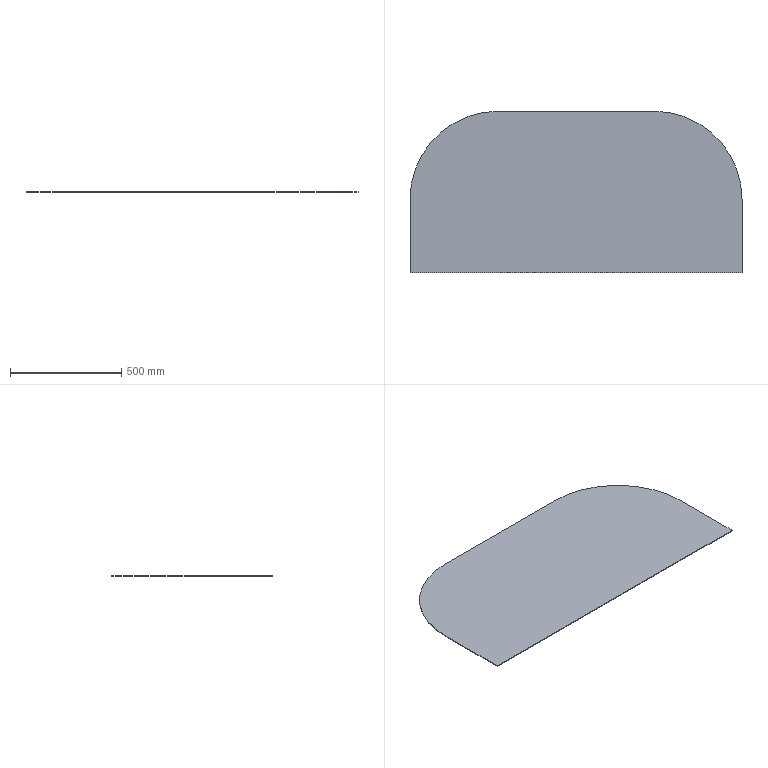Part | NX | features BREP 1, DATUM_CSYS 1, SKETCH 1 | 1 solid | 8 faces | box 1492 x 726 x 3 mm | volume 3047658 mm3 | plane 6 | cylinder 2 | commonest cylinder face diameters 792 x2
STEP:
#1=CARTESIAN_POINT('',(-350.,396.,-1.5));
#2=VERTEX_POINT('',#1);
#3=CARTESIAN_POINT('',(-746.,0.,-1.5));
#4=VERTEX_POINT('',#3);
#5=CARTESIAN_POINT('',(-350.,0.,-1.5));
#6=DIRECTION('',(0.,0.,1.));
#7=DIRECTION('',(1.,0.,0.));
#8=AXIS2_PLACEMENT_3D('',#5,#6,#7);
#9=CIRCLE('',#8,396.);
#10=EDGE_CURVE('',#2,#4,#9,.T.);
#11=ORIENTED_EDGE('',*,*,#10,.T.);
#12=CARTESIAN_POINT('',(-746.,0.,1.5));
#13=VERTEX_POINT('',#12);
#14=CARTESIAN_POINT('',(-746.,0.,1.5));
#15=DIRECTION('',(0.,0.,-1.));
#16=VECTOR('',#15,1000.);
#17=LINE('',#14,#16);
#18=EDGE_CURVE('',#13,#4,#17,.T.);
#19=ORIENTED_EDGE('',*,*,#18,.F.);
#20=CARTESIAN_POINT('',(-350.,396.,1.5));
#21=VERTEX_POINT('',#20);
#22=CARTESIAN_POINT('',(-350.,0.,1.5));
#23=DIRECTION('',(0.,0.,1.));
#24=DIRECTION('',(1.,0.,0.));
#25=AXIS2_PLACEMENT_3D('',#22,#23,#24);
#26=CIRCLE('',#25,396.);
#27=EDGE_CURVE('',#21,#13,#26,.T.);
#28=ORIENTED_EDGE('',*,*,#27,.F.);
#29=CARTESIAN_POINT('',(-350.,396.,1.5));
#30=DIRECTION('',(0.,0.,-1.));
#31=VECTOR('',#30,1000.);
#32=LINE('',#29,#31);
#33=EDGE_CURVE('',#21,#2,#32,.T.);
#34=ORIENTED_EDGE('',*,*,#33,.T.);
#35=EDGE_LOOP('',(#11,#19,#28,#34));
#36=FACE_BOUND('',#35,.T.);
#37=CARTESIAN_POINT('',(-350.,0.,1.5));
#38=DIRECTION('',(0.,0.,-1.));
#39=DIRECTION('',(1.,0.,0.));
#40=AXIS2_PLACEMENT_3D('',#37,#38,#39);
#41=CYLINDRICAL_SURFACE('',#40,396.);
#42=ADVANCED_FACE('',(#36),#41,.T.);
#43=CARTESIAN_POINT('',(-746.,-330.,-1.5));
#44=VERTEX_POINT('',#43);
#45=CARTESIAN_POINT('',(-746.,0.,-1.5));
#46=DIRECTION('',(0.,-1.,0.));
#47=VECTOR('',#46,1000.);
#48=LINE('',#45,#47);
#49=EDGE_CURVE('',#4,#44,#48,.T.);
#50=ORIENTED_EDGE('',*,*,#49,.T.);
#51=CARTESIAN_POINT('',(-746.,-330.,1.5));
#52=VERTEX_POINT('',#51);
#53=CARTESIAN_POINT('',(-746.,-330.,1.5));
#54=DIRECTION('',(0.,0.,-1.));
#55=VECTOR('',#54,1000.);
#56=LINE('',#53,#55);
#57=EDGE_CURVE('',#52,#44,#56,.T.);
#58=ORIENTED_EDGE('',*,*,#57,.F.);
#59=CARTESIAN_POINT('',(-746.,0.,1.5));
#60=DIRECTION('',(0.,-1.,0.));
#61=VECTOR('',#60,1000.);
#62=LINE('',#59,#61);
#63=EDGE_CURVE('',#13,#52,#62,.T.);
#64=ORIENTED_EDGE('',*,*,#63,.F.);
#65=ORIENTED_EDGE('',*,*,#18,.T.);
#66=EDGE_LOOP('',(#50,#58,#64,#65));
#67=FACE_BOUND('',#66,.T.);
#68=CARTESIAN_POINT('',(-746.,0.,1.5));
#69=DIRECTION('',(1.,0.,0.));
#70=DIRECTION('',(0.,-1.,0.));
#71=AXIS2_PLACEMENT_3D('',#68,#69,#70);
#72=PLANE('',#71);
#73=ADVANCED_FACE('',(#67),#72,.F.);
#74=CARTESIAN_POINT('',(746.,-330.,-1.5));
#75=VERTEX_POINT('',#74);
#76=CARTESIAN_POINT('',(-746.,-330.,-1.5));
#77=DIRECTION('',(1.,0.,0.));
#78=VECTOR('',#77,1000.);
#79=LINE('',#76,#78);
#80=EDGE_CURVE('',#44,#75,#79,.T.);
#81=ORIENTED_EDGE('',*,*,#80,.T.);
#82=CARTESIAN_POINT('',(746.,-330.,1.5));
#83=VERTEX_POINT('',#82);
#84=CARTESIAN_POINT('',(746.,-330.,1.5));
#85=DIRECTION('',(0.,0.,-1.));
#86=VECTOR('',#85,1000.);
#87=LINE('',#84,#86);
#88=EDGE_CURVE('',#83,#75,#87,.T.);
#89=ORIENTED_EDGE('',*,*,#88,.F.);
#90=CARTESIAN_POINT('',(-746.,-330.,1.5));
#91=DIRECTION('',(1.,0.,0.));
#92=VECTOR('',#91,1000.);
#93=LINE('',#90,#92);
#94=EDGE_CURVE('',#52,#83,#93,.T.);
#95=ORIENTED_EDGE('',*,*,#94,.F.);
#96=ORIENTED_EDGE('',*,*,#57,.T.);
#97=EDGE_LOOP('',(#81,#89,#95,#96));
#98=FACE_BOUND('',#97,.T.);
#99=CARTESIAN_POINT('',(-746.,-330.,1.5));
#100=DIRECTION('',(0.,1.,0.));
#101=DIRECTION('',(1.,0.,0.));
#102=AXIS2_PLACEMENT_3D('',#99,#100,#101);
#103=PLANE('',#102);
#104=ADVANCED_FACE('',(#98),#103,.F.);
#105=CARTESIAN_POINT('',(746.,0.,-1.5));
#106=VERTEX_POINT('',#105);
#107=CARTESIAN_POINT('',(746.,0.,-1.5));
#108=DIRECTION('',(0.,1.,0.));
#109=VECTOR('',#108,1000.);
#110=LINE('',#107,#109);
#111=EDGE_CURVE('',#75,#106,#110,.T.);
#112=ORIENTED_EDGE('',*,*,#111,.T.);
#113=CARTESIAN_POINT('',(746.,0.,1.5));
#114=VERTEX_POINT('',#113);
#115=CARTESIAN_POINT('',(746.,0.,1.5));
#116=DIRECTION('',(0.,0.,-1.));
#117=VECTOR('',#116,1000.);
#118=LINE('',#115,#117);
#119=EDGE_CURVE('',#114,#106,#118,.T.);
#120=ORIENTED_EDGE('',*,*,#119,.F.);
#121=CARTESIAN_POINT('',(746.,0.,1.5));
#122=DIRECTION('',(0.,1.,0.));
#123=VECTOR('',#122,1000.);
#124=LINE('',#121,#123);
#125=EDGE_CURVE('',#83,#114,#124,.T.);
#126=ORIENTED_EDGE('',*,*,#125,.F.);
#127=ORIENTED_EDGE('',*,*,#88,.T.);
#128=EDGE_LOOP('',(#112,#120,#126,#127));
#129=FACE_BOUND('',#128,.T.);
#130=CARTESIAN_POINT('',(746.,0.,1.5));
#131=DIRECTION('',(-1.,0.,0.));
#132=DIRECTION('',(0.,1.,0.));
#133=AXIS2_PLACEMENT_3D('',#130,#131,#132);
#134=PLANE('',#133);
#135=ADVANCED_FACE('',(#129),#134,.F.);
#136=CARTESIAN_POINT('',(350.,396.,-1.5));
#137=VERTEX_POINT('',#136);
#138=CARTESIAN_POINT('',(350.,0.,-1.5));
#139=DIRECTION('',(0.,0.,1.));
#140=DIRECTION('',(-1.,0.,0.));
#141=AXIS2_PLACEMENT_3D('',#138,#139,#140);
#142=CIRCLE('',#141,396.);
#143=EDGE_CURVE('',#106,#137,#142,.T.);
#144=ORIENTED_EDGE('',*,*,#143,.T.);
#145=CARTESIAN_POINT('',(350.,396.,1.5));
#146=VERTEX_POINT('',#145);
#147=CARTESIAN_POINT('',(350.,396.,1.5));
#148=DIRECTION('',(0.,0.,-1.));
#149=VECTOR('',#148,1000.);
#150=LINE('',#147,#149);
#151=EDGE_CURVE('',#146,#137,#150,.T.);
#152=ORIENTED_EDGE('',*,*,#151,.F.);
#153=CARTESIAN_POINT('',(350.,0.,1.5));
#154=DIRECTION('',(0.,0.,1.));
#155=DIRECTION('',(-1.,0.,0.));
#156=AXIS2_PLACEMENT_3D('',#153,#154,#155);
#157=CIRCLE('',#156,396.);
#158=EDGE_CURVE('',#114,#146,#157,.T.);
#159=ORIENTED_EDGE('',*,*,#158,.F.);
#160=ORIENTED_EDGE('',*,*,#119,.T.);
#161=EDGE_LOOP('',(#144,#152,#159,#160));
#162=FACE_BOUND('',#161,.T.);
#163=CARTESIAN_POINT('',(350.,0.,1.5));
#164=DIRECTION('',(0.,0.,-1.));
#165=DIRECTION('',(1.,0.,0.));
#166=AXIS2_PLACEMENT_3D('',#163,#164,#165);
#167=CYLINDRICAL_SURFACE('',#166,396.);
#168=ADVANCED_FACE('',(#162),#167,.T.);
#169=CARTESIAN_POINT('',(-350.,396.,-1.5));
#170=DIRECTION('',(-1.,0.,0.));
#171=VECTOR('',#170,1000.);
#172=LINE('',#169,#171);
#173=EDGE_CURVE('',#137,#2,#172,.T.);
#174=ORIENTED_EDGE('',*,*,#173,.T.);
#175=ORIENTED_EDGE('',*,*,#33,.F.);
#176=CARTESIAN_POINT('',(-350.,396.,1.5));
#177=DIRECTION('',(-1.,0.,0.));
#178=VECTOR('',#177,1000.);
#179=LINE('',#176,#178);
#180=EDGE_CURVE('',#146,#21,#179,.T.);
#181=ORIENTED_EDGE('',*,*,#180,.F.);
#182=ORIENTED_EDGE('',*,*,#151,.T.);
#183=EDGE_LOOP('',(#174,#175,#181,#182));
#184=FACE_BOUND('',#183,.T.);
#185=CARTESIAN_POINT('',(-350.,396.,1.5));
#186=DIRECTION('',(0.,-1.,0.));
#187=DIRECTION('',(-1.,0.,0.));
#188=AXIS2_PLACEMENT_3D('',#185,#186,#187);
#189=PLANE('',#188);
#190=ADVANCED_FACE('',(#184),#189,.F.);
#191=ORIENTED_EDGE('',*,*,#27,.T.);
#192=ORIENTED_EDGE('',*,*,#63,.T.);
#193=ORIENTED_EDGE('',*,*,#94,.T.);
#194=ORIENTED_EDGE('',*,*,#125,.T.);
#195=ORIENTED_EDGE('',*,*,#158,.T.);
#196=ORIENTED_EDGE('',*,*,#180,.T.);
#197=EDGE_LOOP('',(#191,#192,#193,#194,#195,#196));
#198=FACE_BOUND('',#197,.T.);
#199=CARTESIAN_POINT('',(-350.,0.,1.5));
#200=DIRECTION('',(0.,0.,1.));
#201=DIRECTION('',(-1.,0.,0.));
#202=AXIS2_PLACEMENT_3D('',#199,#200,#201);
#203=PLANE('',#202);
#204=ADVANCED_FACE('',(#198),#203,.T.);
#205=ORIENTED_EDGE('',*,*,#10,.F.);
#206=ORIENTED_EDGE('',*,*,#173,.F.);
#207=ORIENTED_EDGE('',*,*,#143,.F.);
#208=ORIENTED_EDGE('',*,*,#111,.F.);
#209=ORIENTED_EDGE('',*,*,#80,.F.);
#210=ORIENTED_EDGE('',*,*,#49,.F.);
#211=EDGE_LOOP('',(#205,#206,#207,#208,#209,#210));
#212=FACE_BOUND('',#211,.T.);
#213=CARTESIAN_POINT('',(-350.,0.,-1.5));
#214=DIRECTION('',(0.,0.,1.));
#215=DIRECTION('',(-1.,0.,0.));
#216=AXIS2_PLACEMENT_3D('',#213,#214,#215);
#217=PLANE('',#216);
#218=ADVANCED_FACE('',(#212),#217,.F.);
#219=CLOSED_SHELL('',(#42,#73,#104,#135,#168,#190,#204,#218));
#220=MANIFOLD_SOLID_BREP('',#219);
#221=(LENGTH_UNIT()NAMED_UNIT(*)SI_UNIT(.MILLI.,.METRE.));
#222=UNCERTAINTY_MEASURE_WITH_UNIT(LENGTH_MEASURE(0.00001),#221,'','');
#223=(NAMED_UNIT(*)PLANE_ANGLE_UNIT()SI_UNIT($,.RADIAN.));
#224=(NAMED_UNIT(*)SI_UNIT($,.STERADIAN.)SOLID_ANGLE_UNIT());
#225=(GEOMETRIC_REPRESENTATION_CONTEXT(3)GLOBAL_UNCERTAINTY_ASSIGNED_CONTEXT((#222))GLOBAL_UNIT_ASSIGNED_CONTEXT((#221,#223,#224))REPRESENTATION_CONTEXT('',''));
#226=ADVANCED_BREP_SHAPE_REPRESENTATION('',(#220),#225);